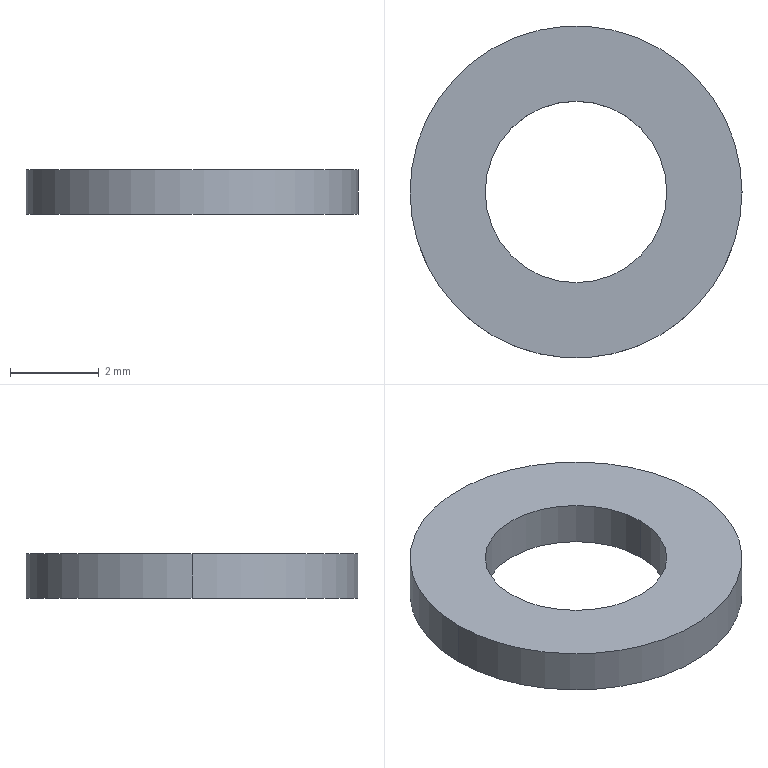Part | STEP file | 11-FG-SZ01211 | 1 solid | 6 faces | box 7.5 x 7.5 x 1 mm | volume 30.976 mm3 | cylinder 4 | plane 2 | commonest cylinder face diameters 4.1 x2 7.5 x2
STEP:
#1=CARTESIAN_POINT('',(-89.13,-247.716,1.));
#2=VERTEX_POINT('',#1);
#3=CARTESIAN_POINT('',(-85.03,-247.716,1.));
#4=VERTEX_POINT('',#3);
#5=CARTESIAN_POINT('',(-87.08,-247.716,1.));
#6=DIRECTION('',(0.,0.,1.));
#7=DIRECTION('',(1.,0.,0.));
#8=AXIS2_PLACEMENT_3D('',#5,#6,#7);
#9=CIRCLE('',#8,2.05);
#10=EDGE_CURVE('',#2,#4,#9,.T.);
#11=ORIENTED_EDGE('',*,*,#10,.T.);
#12=CARTESIAN_POINT('',(-85.03,-247.716,0.));
#13=VERTEX_POINT('',#12);
#14=CARTESIAN_POINT('',(-85.03,-247.716,1.));
#15=DIRECTION('',(0.,0.,-1.));
#16=VECTOR('',#15,1000.);
#17=LINE('',#14,#16);
#18=EDGE_CURVE('',#4,#13,#17,.T.);
#19=ORIENTED_EDGE('',*,*,#18,.T.);
#20=CARTESIAN_POINT('',(-89.13,-247.716,0.));
#21=VERTEX_POINT('',#20);
#22=CARTESIAN_POINT('',(-87.08,-247.716,0.));
#23=DIRECTION('',(0.,0.,1.));
#24=DIRECTION('',(1.,0.,0.));
#25=AXIS2_PLACEMENT_3D('',#22,#23,#24);
#26=CIRCLE('',#25,2.05);
#27=EDGE_CURVE('',#21,#13,#26,.T.);
#28=ORIENTED_EDGE('',*,*,#27,.F.);
#29=CARTESIAN_POINT('',(-89.13,-247.716,1.));
#30=DIRECTION('',(0.,0.,-1.));
#31=VECTOR('',#30,1000.);
#32=LINE('',#29,#31);
#33=EDGE_CURVE('',#2,#21,#32,.T.);
#34=ORIENTED_EDGE('',*,*,#33,.F.);
#35=EDGE_LOOP('',(#11,#19,#28,#34));
#36=FACE_OUTER_BOUND('',#35,.T.);
#37=CARTESIAN_POINT('',(-87.08,-247.716,1.));
#38=DIRECTION('',(0.,0.,-1.));
#39=DIRECTION('',(-1.,0.,0.));
#40=AXIS2_PLACEMENT_3D('',#37,#38,#39);
#41=CYLINDRICAL_SURFACE('',#40,2.05);
#42=ADVANCED_FACE('',(#36),#41,.F.);
#43=CARTESIAN_POINT('',(-83.33,-247.716,1.));
#44=VERTEX_POINT('',#43);
#45=CARTESIAN_POINT('',(-90.83,-247.716,1.));
#46=VERTEX_POINT('',#45);
#47=CARTESIAN_POINT('',(-87.08,-247.716,1.));
#48=DIRECTION('',(0.,0.,1.));
#49=DIRECTION('',(1.,0.,0.));
#50=AXIS2_PLACEMENT_3D('',#47,#48,#49);
#51=CIRCLE('',#50,3.75);
#52=EDGE_CURVE('',#44,#46,#51,.T.);
#53=ORIENTED_EDGE('',*,*,#52,.F.);
#54=CARTESIAN_POINT('',(-83.33,-247.716,0.));
#55=VERTEX_POINT('',#54);
#56=CARTESIAN_POINT('',(-83.33,-247.716,1.));
#57=DIRECTION('',(0.,0.,-1.));
#58=VECTOR('',#57,1000.);
#59=LINE('',#56,#58);
#60=EDGE_CURVE('',#44,#55,#59,.T.);
#61=ORIENTED_EDGE('',*,*,#60,.T.);
#62=CARTESIAN_POINT('',(-90.83,-247.716,0.));
#63=VERTEX_POINT('',#62);
#64=CARTESIAN_POINT('',(-87.08,-247.716,0.));
#65=DIRECTION('',(0.,0.,1.));
#66=DIRECTION('',(1.,0.,0.));
#67=AXIS2_PLACEMENT_3D('',#64,#65,#66);
#68=CIRCLE('',#67,3.75);
#69=EDGE_CURVE('',#55,#63,#68,.T.);
#70=ORIENTED_EDGE('',*,*,#69,.T.);
#71=CARTESIAN_POINT('',(-90.83,-247.716,1.));
#72=DIRECTION('',(0.,0.,-1.));
#73=VECTOR('',#72,1000.);
#74=LINE('',#71,#73);
#75=EDGE_CURVE('',#46,#63,#74,.T.);
#76=ORIENTED_EDGE('',*,*,#75,.F.);
#77=EDGE_LOOP('',(#53,#61,#70,#76));
#78=FACE_OUTER_BOUND('',#77,.T.);
#79=CARTESIAN_POINT('',(-87.08,-247.716,1.));
#80=DIRECTION('',(0.,0.,-1.));
#81=DIRECTION('',(-1.,0.,0.));
#82=AXIS2_PLACEMENT_3D('',#79,#80,#81);
#83=CYLINDRICAL_SURFACE('',#82,3.75);
#84=ADVANCED_FACE('',(#78),#83,.T.);
#85=CARTESIAN_POINT('',(-87.08,-247.716,1.));
#86=DIRECTION('',(0.,0.,1.));
#87=DIRECTION('',(1.,0.,0.));
#88=AXIS2_PLACEMENT_3D('',#85,#86,#87);
#89=CIRCLE('',#88,3.75);
#90=EDGE_CURVE('',#46,#44,#89,.T.);
#91=ORIENTED_EDGE('',*,*,#90,.T.);
#92=ORIENTED_EDGE('',*,*,#52,.T.);
#93=EDGE_LOOP('',(#91,#92));
#94=FACE_OUTER_BOUND('',#93,.T.);
#95=ORIENTED_EDGE('',*,*,#10,.F.);
#96=CARTESIAN_POINT('',(-87.08,-247.716,1.));
#97=DIRECTION('',(0.,0.,1.));
#98=DIRECTION('',(1.,0.,0.));
#99=AXIS2_PLACEMENT_3D('',#96,#97,#98);
#100=CIRCLE('',#99,2.05);
#101=EDGE_CURVE('',#4,#2,#100,.T.);
#102=ORIENTED_EDGE('',*,*,#101,.F.);
#103=EDGE_LOOP('',(#95,#102));
#104=FACE_BOUND('',#103,.T.);
#105=CARTESIAN_POINT('',(-87.08,-247.716,1.));
#106=DIRECTION('',(0.,0.,1.));
#107=DIRECTION('',(1.,0.,0.));
#108=AXIS2_PLACEMENT_3D('',#105,#106,#107);
#109=PLANE('',#108);
#110=ADVANCED_FACE('',(#94,#104),#109,.T.);
#111=CARTESIAN_POINT('',(-87.08,-247.716,0.));
#112=DIRECTION('',(0.,0.,1.));
#113=DIRECTION('',(1.,0.,0.));
#114=AXIS2_PLACEMENT_3D('',#111,#112,#113);
#115=CIRCLE('',#114,3.75);
#116=EDGE_CURVE('',#63,#55,#115,.T.);
#117=ORIENTED_EDGE('',*,*,#116,.F.);
#118=ORIENTED_EDGE('',*,*,#69,.F.);
#119=EDGE_LOOP('',(#117,#118));
#120=FACE_OUTER_BOUND('',#119,.T.);
#121=ORIENTED_EDGE('',*,*,#27,.T.);
#122=CARTESIAN_POINT('',(-87.08,-247.716,0.));
#123=DIRECTION('',(0.,0.,1.));
#124=DIRECTION('',(1.,0.,0.));
#125=AXIS2_PLACEMENT_3D('',#122,#123,#124);
#126=CIRCLE('',#125,2.05);
#127=EDGE_CURVE('',#13,#21,#126,.T.);
#128=ORIENTED_EDGE('',*,*,#127,.T.);
#129=EDGE_LOOP('',(#121,#128));
#130=FACE_BOUND('',#129,.T.);
#131=CARTESIAN_POINT('',(-87.08,-247.716,0.));
#132=DIRECTION('',(0.,0.,1.));
#133=DIRECTION('',(1.,0.,0.));
#134=AXIS2_PLACEMENT_3D('',#131,#132,#133);
#135=PLANE('',#134);
#136=ADVANCED_FACE('',(#120,#130),#135,.F.);
#137=ORIENTED_EDGE('',*,*,#60,.F.);
#138=ORIENTED_EDGE('',*,*,#90,.F.);
#139=ORIENTED_EDGE('',*,*,#75,.T.);
#140=ORIENTED_EDGE('',*,*,#116,.T.);
#141=EDGE_LOOP('',(#137,#138,#139,#140));
#142=FACE_OUTER_BOUND('',#141,.T.);
#143=CARTESIAN_POINT('',(-87.08,-247.716,1.));
#144=DIRECTION('',(0.,0.,-1.));
#145=DIRECTION('',(-1.,0.,0.));
#146=AXIS2_PLACEMENT_3D('',#143,#144,#145);
#147=CYLINDRICAL_SURFACE('',#146,3.75);
#148=ADVANCED_FACE('',(#142),#147,.T.);
#149=ORIENTED_EDGE('',*,*,#18,.F.);
#150=ORIENTED_EDGE('',*,*,#101,.T.);
#151=ORIENTED_EDGE('',*,*,#33,.T.);
#152=ORIENTED_EDGE('',*,*,#127,.F.);
#153=EDGE_LOOP('',(#149,#150,#151,#152));
#154=FACE_OUTER_BOUND('',#153,.T.);
#155=CARTESIAN_POINT('',(-87.08,-247.716,1.));
#156=DIRECTION('',(0.,0.,-1.));
#157=DIRECTION('',(-1.,0.,0.));
#158=AXIS2_PLACEMENT_3D('',#155,#156,#157);
#159=CYLINDRICAL_SURFACE('',#158,2.05);
#160=ADVANCED_FACE('',(#154),#159,.F.);
#161=CLOSED_SHELL('',(#42,#84,#110,#136,#148,#160));
#162=MANIFOLD_SOLID_BREP('',#161);
#163=CARTESIAN_POINT('',(0.,0.,0.));
#164=DIRECTION('',(0.,0.,1.));
#165=DIRECTION('',(1.,0.,0.));
#166=AXIS2_PLACEMENT_3D('',#163,#164,#165);
#167=(LENGTH_UNIT()NAMED_UNIT(*)SI_UNIT(.MILLI.,.METRE.));
#168=UNCERTAINTY_MEASURE_WITH_UNIT(LENGTH_MEASURE(0.00001),#167,'','');
#169=(NAMED_UNIT(*)PLANE_ANGLE_UNIT()SI_UNIT($,.RADIAN.));
#170=(NAMED_UNIT(*)SI_UNIT($,.STERADIAN.)SOLID_ANGLE_UNIT());
#171=(GEOMETRIC_REPRESENTATION_CONTEXT(3)GLOBAL_UNCERTAINTY_ASSIGNED_CONTEXT((#168))GLOBAL_UNIT_ASSIGNED_CONTEXT((#167,#169,#170))REPRESENTATION_CONTEXT('',''));
#172=ADVANCED_BREP_SHAPE_REPRESENTATION('',(#162,#166),#171);